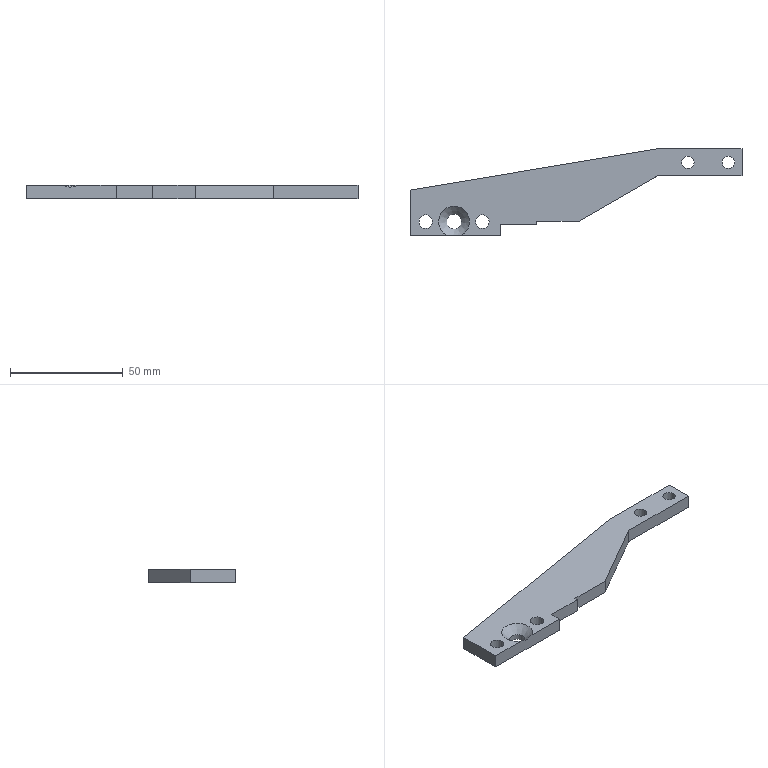Part | NX | features BREP 1 | 1 solid | 19 faces | box 147 x 38.3 x 6 mm | volume 16283 mm3 | plane 13 | cylinder 5 | cone 1 | commonest cylinder face diameters 5.5 x2 6 x2 6.6 x1
STEP:
#1=CARTESIAN_POINT('',(73.5,1.3,-3.));
#2=VERTEX_POINT('',#1);
#3=CARTESIAN_POINT('',(73.5,13.3,-3.));
#4=VERTEX_POINT('',#3);
#5=CARTESIAN_POINT('',(73.5,-25.,-3.));
#6=DIRECTION('',(0.,1.,0.));
#7=VECTOR('',#6,1000.);
#8=LINE('',#5,#7);
#9=EDGE_CURVE('',#2,#4,#8,.T.);
#10=ORIENTED_EDGE('',*,*,#9,.T.);
#11=CARTESIAN_POINT('',(73.5,13.3,3.));
#12=VERTEX_POINT('',#11);
#13=CARTESIAN_POINT('',(73.5,13.3,-153.03));
#14=DIRECTION('',(0.,0.,1.));
#15=VECTOR('',#14,1000.);
#16=LINE('',#13,#15);
#17=EDGE_CURVE('',#4,#12,#16,.T.);
#18=ORIENTED_EDGE('',*,*,#17,.T.);
#19=CARTESIAN_POINT('',(73.5,1.3,3.));
#20=VERTEX_POINT('',#19);
#21=CARTESIAN_POINT('',(73.5,-25.,3.));
#22=DIRECTION('',(0.,1.,0.));
#23=VECTOR('',#22,1000.);
#24=LINE('',#21,#23);
#25=EDGE_CURVE('',#20,#12,#24,.T.);
#26=ORIENTED_EDGE('',*,*,#25,.F.);
#27=CARTESIAN_POINT('',(73.5,1.3,-113.185));
#28=DIRECTION('',(0.,0.,1.));
#29=VECTOR('',#28,1000.);
#30=LINE('',#27,#29);
#31=EDGE_CURVE('',#2,#20,#30,.T.);
#32=ORIENTED_EDGE('',*,*,#31,.F.);
#33=EDGE_LOOP('',(#10,#18,#26,#32));
#34=FACE_BOUND('',#33,.T.);
#35=CARTESIAN_POINT('',(73.5,-25.,3.));
#36=DIRECTION('',(-1.,0.,0.));
#37=DIRECTION('',(0.,0.,-1.));
#38=AXIS2_PLACEMENT_3D('',#35,#36,#37);
#39=PLANE('',#38);
#40=ADVANCED_FACE('',(#34),#39,.F.);
#41=CARTESIAN_POINT('',(-73.5,-5.,3.));
#42=VERTEX_POINT('',#41);
#43=CARTESIAN_POINT('',(-73.5,-25.,3.));
#44=VERTEX_POINT('',#43);
#45=CARTESIAN_POINT('',(-73.5,-25.,3.));
#46=DIRECTION('',(0.,-1.,0.));
#47=VECTOR('',#46,1000.);
#48=LINE('',#45,#47);
#49=EDGE_CURVE('',#42,#44,#48,.T.);
#50=ORIENTED_EDGE('',*,*,#49,.F.);
#51=CARTESIAN_POINT('',(-73.5,-5.,-3.));
#52=VERTEX_POINT('',#51);
#53=CARTESIAN_POINT('',(-73.5,-5.,-153.03));
#54=DIRECTION('',(0.,0.,1.));
#55=VECTOR('',#54,1000.);
#56=LINE('',#53,#55);
#57=EDGE_CURVE('',#52,#42,#56,.T.);
#58=ORIENTED_EDGE('',*,*,#57,.F.);
#59=CARTESIAN_POINT('',(-73.5,-25.,-3.));
#60=VERTEX_POINT('',#59);
#61=CARTESIAN_POINT('',(-73.5,-25.,-3.));
#62=DIRECTION('',(0.,-1.,0.));
#63=VECTOR('',#62,1000.);
#64=LINE('',#61,#63);
#65=EDGE_CURVE('',#52,#60,#64,.T.);
#66=ORIENTED_EDGE('',*,*,#65,.T.);
#67=CARTESIAN_POINT('',(-73.5,-25.,3.));
#68=DIRECTION('',(0.,0.,-1.));
#69=VECTOR('',#68,1000.);
#70=LINE('',#67,#69);
#71=EDGE_CURVE('',#44,#60,#70,.T.);
#72=ORIENTED_EDGE('',*,*,#71,.F.);
#73=EDGE_LOOP('',(#50,#58,#66,#72));
#74=FACE_BOUND('',#73,.T.);
#75=CARTESIAN_POINT('',(-73.5,-25.,3.));
#76=DIRECTION('',(1.,0.,0.));
#77=DIRECTION('',(0.,0.,1.));
#78=AXIS2_PLACEMENT_3D('',#75,#76,#77);
#79=PLANE('',#78);
#80=ADVANCED_FACE('',(#74),#79,.F.);
#81=CARTESIAN_POINT('',(-33.5,-25.,-3.));
#82=VERTEX_POINT('',#81);
#83=CARTESIAN_POINT('',(-73.5,-25.,-3.));
#84=DIRECTION('',(1.,0.,0.));
#85=VECTOR('',#84,1000.);
#86=LINE('',#83,#85);
#87=EDGE_CURVE('',#60,#82,#86,.T.);
#88=ORIENTED_EDGE('',*,*,#87,.T.);
#89=CARTESIAN_POINT('',(-33.5,-25.,3.));
#90=VERTEX_POINT('',#89);
#91=CARTESIAN_POINT('',(-33.5,-25.,-113.185));
#92=DIRECTION('',(0.,0.,1.));
#93=VECTOR('',#92,1000.);
#94=LINE('',#91,#93);
#95=EDGE_CURVE('',#82,#90,#94,.T.);
#96=ORIENTED_EDGE('',*,*,#95,.T.);
#97=CARTESIAN_POINT('',(-50.685,-25.,3.));
#98=VERTEX_POINT('',#97);
#99=CARTESIAN_POINT('',(-73.5,-25.,3.));
#100=DIRECTION('',(1.,0.,0.));
#101=VECTOR('',#100,1000.);
#102=LINE('',#99,#101);
#103=EDGE_CURVE('',#98,#90,#102,.T.);
#104=ORIENTED_EDGE('',*,*,#103,.F.);
#105=CARTESIAN_POINT('',(-57.315,-25.,3.));
#106=VERTEX_POINT('',#105);
#107=CARTESIAN_POINT('',(-50.685,-25.,3.));
#108=CARTESIAN_POINT('',(-51.725,-25.,2.497));
#109=CARTESIAN_POINT('',(-53.981,-25.,1.794));
#110=CARTESIAN_POINT('',(-56.27,-25.,2.494));
#111=CARTESIAN_POINT('',(-57.315,-25.,3.));
#112=B_SPLINE_CURVE_WITH_KNOTS('',3,(#107,#108,#109,#110,#111),.UNSPECIFIED.,.F.,.F.,(4,1,4),(0.,0.003417,0.006834),.UNSPECIFIED.);
#113=EDGE_CURVE('',#98,#106,#112,.T.);
#114=ORIENTED_EDGE('',*,*,#113,.T.);
#115=CARTESIAN_POINT('',(-73.5,-25.,3.));
#116=DIRECTION('',(1.,0.,0.));
#117=VECTOR('',#116,1000.);
#118=LINE('',#115,#117);
#119=EDGE_CURVE('',#44,#106,#118,.T.);
#120=ORIENTED_EDGE('',*,*,#119,.F.);
#121=ORIENTED_EDGE('',*,*,#71,.T.);
#122=EDGE_LOOP('',(#88,#96,#104,#114,#120,#121));
#123=FACE_BOUND('',#122,.T.);
#124=CARTESIAN_POINT('',(-73.5,-25.,3.));
#125=DIRECTION('',(0.,1.,0.));
#126=DIRECTION('',(0.,0.,-1.));
#127=AXIS2_PLACEMENT_3D('',#124,#125,#126);
#128=PLANE('',#127);
#129=ADVANCED_FACE('',(#123),#128,.F.);
#130=CARTESIAN_POINT('',(52.25,7.3,3.));
#131=VERTEX_POINT('',#130);
#132=CARTESIAN_POINT('',(49.5,7.3,3.));
#133=DIRECTION('',(0.,0.,1.));
#134=DIRECTION('',(1.,0.,0.));
#135=AXIS2_PLACEMENT_3D('',#132,#133,#134);
#136=CIRCLE('',#135,2.75);
#137=EDGE_CURVE('',#131,#131,#136,.T.);
#138=ORIENTED_EDGE('',*,*,#137,.F.);
#139=EDGE_LOOP('',(#138));
#140=FACE_BOUND('',#139,.T.);
#141=CARTESIAN_POINT('',(70.25,7.3,3.));
#142=VERTEX_POINT('',#141);
#143=CARTESIAN_POINT('',(67.5,7.3,3.));
#144=DIRECTION('',(0.,0.,1.));
#145=DIRECTION('',(1.,0.,0.));
#146=AXIS2_PLACEMENT_3D('',#143,#144,#145);
#147=CIRCLE('',#146,2.75);
#148=EDGE_CURVE('',#142,#142,#147,.T.);
#149=ORIENTED_EDGE('',*,*,#148,.F.);
#150=EDGE_LOOP('',(#149));
#151=FACE_BOUND('',#150,.T.);
#152=CARTESIAN_POINT('',(-63.5,-19.,3.));
#153=VERTEX_POINT('',#152);
#154=CARTESIAN_POINT('',(-66.5,-19.,3.));
#155=DIRECTION('',(0.,0.,1.));
#156=DIRECTION('',(1.,0.,0.));
#157=AXIS2_PLACEMENT_3D('',#154,#155,#156);
#158=CIRCLE('',#157,3.);
#159=EDGE_CURVE('',#153,#153,#158,.T.);
#160=ORIENTED_EDGE('',*,*,#159,.F.);
#161=EDGE_LOOP('',(#160));
#162=FACE_BOUND('',#161,.T.);
#163=CARTESIAN_POINT('',(-38.5,-19.,3.));
#164=VERTEX_POINT('',#163);
#165=CARTESIAN_POINT('',(-41.5,-19.,3.));
#166=DIRECTION('',(0.,0.,1.));
#167=DIRECTION('',(1.,0.,0.));
#168=AXIS2_PLACEMENT_3D('',#165,#166,#167);
#169=CIRCLE('',#168,3.);
#170=EDGE_CURVE('',#164,#164,#169,.T.);
#171=ORIENTED_EDGE('',*,*,#170,.F.);
#172=EDGE_LOOP('',(#171));
#173=FACE_BOUND('',#172,.T.);
#174=CARTESIAN_POINT('',(36.141,13.3,3.));
#175=VERTEX_POINT('',#174);
#176=CARTESIAN_POINT('',(36.141,13.3,3.));
#177=DIRECTION('',(1.,0.,0.));
#178=VECTOR('',#177,1000.);
#179=LINE('',#176,#178);
#180=EDGE_CURVE('',#175,#12,#179,.T.);
#181=ORIENTED_EDGE('',*,*,#180,.F.);
#182=CARTESIAN_POINT('',(-73.5,-5.,3.));
#183=DIRECTION('',(0.9864,0.1646,0.));
#184=VECTOR('',#183,1000.);
#185=LINE('',#182,#184);
#186=EDGE_CURVE('',#42,#175,#185,.T.);
#187=ORIENTED_EDGE('',*,*,#186,.F.);
#188=ORIENTED_EDGE('',*,*,#49,.T.);
#189=ORIENTED_EDGE('',*,*,#119,.T.);
#190=CARTESIAN_POINT('',(-54.,-19.,3.));
#191=DIRECTION('',(0.,0.,1.));
#192=DIRECTION('',(1.,0.,0.));
#193=AXIS2_PLACEMENT_3D('',#190,#191,#192);
#194=CIRCLE('',#193,6.855);
#195=EDGE_CURVE('',#98,#106,#194,.T.);
#196=ORIENTED_EDGE('',*,*,#195,.F.);
#197=ORIENTED_EDGE('',*,*,#103,.T.);
#198=CARTESIAN_POINT('',(-33.5,-20.1,3.));
#199=VERTEX_POINT('',#198);
#200=CARTESIAN_POINT('',(-33.5,-25.,3.));
#201=DIRECTION('',(0.,-1.,0.));
#202=VECTOR('',#201,1000.);
#203=LINE('',#200,#202);
#204=EDGE_CURVE('',#199,#90,#203,.T.);
#205=ORIENTED_EDGE('',*,*,#204,.F.);
#206=CARTESIAN_POINT('',(-17.5,-20.1,3.));
#207=VERTEX_POINT('',#206);
#208=CARTESIAN_POINT('',(-33.5,-20.1,3.));
#209=DIRECTION('',(1.,0.,0.));
#210=VECTOR('',#209,1000.);
#211=LINE('',#208,#210);
#212=EDGE_CURVE('',#199,#207,#211,.T.);
#213=ORIENTED_EDGE('',*,*,#212,.T.);
#214=CARTESIAN_POINT('',(-17.5,-18.7,3.));
#215=VERTEX_POINT('',#214);
#216=CARTESIAN_POINT('',(-17.5,-18.7,3.));
#217=DIRECTION('',(0.,1.,0.));
#218=VECTOR('',#217,1000.);
#219=LINE('',#216,#218);
#220=EDGE_CURVE('',#207,#215,#219,.T.);
#221=ORIENTED_EDGE('',*,*,#220,.T.);
#222=CARTESIAN_POINT('',(1.5,-18.7,3.));
#223=VERTEX_POINT('',#222);
#224=CARTESIAN_POINT('',(-33.5,-18.7,3.));
#225=DIRECTION('',(-1.,0.,0.));
#226=VECTOR('',#225,1000.);
#227=LINE('',#224,#226);
#228=EDGE_CURVE('',#223,#215,#227,.T.);
#229=ORIENTED_EDGE('',*,*,#228,.F.);
#230=CARTESIAN_POINT('',(36.141,1.3,3.));
#231=VERTEX_POINT('',#230);
#232=CARTESIAN_POINT('',(1.5,-18.7,3.));
#233=DIRECTION('',(-0.866,-0.5,0.));
#234=VECTOR('',#233,1000.);
#235=LINE('',#232,#234);
#236=EDGE_CURVE('',#231,#223,#235,.T.);
#237=ORIENTED_EDGE('',*,*,#236,.F.);
#238=CARTESIAN_POINT('',(36.141,1.3,3.));
#239=DIRECTION('',(-1.,0.,0.));
#240=VECTOR('',#239,1000.);
#241=LINE('',#238,#240);
#242=EDGE_CURVE('',#20,#231,#241,.T.);
#243=ORIENTED_EDGE('',*,*,#242,.F.);
#244=ORIENTED_EDGE('',*,*,#25,.T.);
#245=EDGE_LOOP('',(#181,#187,#188,#189,#196,#197,#205,#213,#221,#229,#237,#243,#244));
#246=FACE_BOUND('',#245,.T.);
#247=CARTESIAN_POINT('',(0.,0.,3.));
#248=DIRECTION('',(0.,0.,-1.));
#249=DIRECTION('',(1.,0.,0.));
#250=AXIS2_PLACEMENT_3D('',#247,#248,#249);
#251=PLANE('',#250);
#252=ADVANCED_FACE('',(#140,#151,#162,#173,#246),#251,.F.);
#253=CARTESIAN_POINT('',(46.75,7.3,-3.));
#254=VERTEX_POINT('',#253);
#255=CARTESIAN_POINT('',(49.5,7.3,-3.));
#256=DIRECTION('',(0.,0.,-1.));
#257=DIRECTION('',(-1.,0.,0.));
#258=AXIS2_PLACEMENT_3D('',#255,#256,#257);
#259=CIRCLE('',#258,2.75);
#260=EDGE_CURVE('',#254,#254,#259,.T.);
#261=ORIENTED_EDGE('',*,*,#260,.F.);
#262=EDGE_LOOP('',(#261));
#263=FACE_BOUND('',#262,.T.);
#264=CARTESIAN_POINT('',(64.75,7.3,-3.));
#265=VERTEX_POINT('',#264);
#266=CARTESIAN_POINT('',(67.5,7.3,-3.));
#267=DIRECTION('',(0.,0.,-1.));
#268=DIRECTION('',(-1.,0.,0.));
#269=AXIS2_PLACEMENT_3D('',#266,#267,#268);
#270=CIRCLE('',#269,2.75);
#271=EDGE_CURVE('',#265,#265,#270,.T.);
#272=ORIENTED_EDGE('',*,*,#271,.F.);
#273=EDGE_LOOP('',(#272));
#274=FACE_BOUND('',#273,.T.);
#275=CARTESIAN_POINT('',(36.141,13.3,-3.));
#276=VERTEX_POINT('',#275);
#277=CARTESIAN_POINT('',(-73.5,-5.,-3.));
#278=DIRECTION('',(0.9864,0.1646,0.));
#279=VECTOR('',#278,1000.);
#280=LINE('',#277,#279);
#281=EDGE_CURVE('',#52,#276,#280,.T.);
#282=ORIENTED_EDGE('',*,*,#281,.T.);
#283=CARTESIAN_POINT('',(36.141,13.3,-3.));
#284=DIRECTION('',(1.,0.,0.));
#285=VECTOR('',#284,1000.);
#286=LINE('',#283,#285);
#287=EDGE_CURVE('',#276,#4,#286,.T.);
#288=ORIENTED_EDGE('',*,*,#287,.T.);
#289=ORIENTED_EDGE('',*,*,#9,.F.);
#290=CARTESIAN_POINT('',(36.141,1.3,-3.));
#291=VERTEX_POINT('',#290);
#292=CARTESIAN_POINT('',(36.141,1.3,-3.));
#293=DIRECTION('',(-1.,0.,0.));
#294=VECTOR('',#293,1000.);
#295=LINE('',#292,#294);
#296=EDGE_CURVE('',#2,#291,#295,.T.);
#297=ORIENTED_EDGE('',*,*,#296,.T.);
#298=CARTESIAN_POINT('',(1.5,-18.7,-3.));
#299=VERTEX_POINT('',#298);
#300=CARTESIAN_POINT('',(1.5,-18.7,-3.));
#301=DIRECTION('',(-0.866,-0.5,0.));
#302=VECTOR('',#301,1000.);
#303=LINE('',#300,#302);
#304=EDGE_CURVE('',#291,#299,#303,.T.);
#305=ORIENTED_EDGE('',*,*,#304,.T.);
#306=CARTESIAN_POINT('',(-17.5,-18.7,-3.));
#307=VERTEX_POINT('',#306);
#308=CARTESIAN_POINT('',(-33.5,-18.7,-3.));
#309=DIRECTION('',(-1.,0.,0.));
#310=VECTOR('',#309,1000.);
#311=LINE('',#308,#310);
#312=EDGE_CURVE('',#299,#307,#311,.T.);
#313=ORIENTED_EDGE('',*,*,#312,.T.);
#314=CARTESIAN_POINT('',(-17.5,-20.1,-3.));
#315=VERTEX_POINT('',#314);
#316=CARTESIAN_POINT('',(-17.5,-18.7,-3.));
#317=DIRECTION('',(0.,1.,0.));
#318=VECTOR('',#317,1000.);
#319=LINE('',#316,#318);
#320=EDGE_CURVE('',#315,#307,#319,.T.);
#321=ORIENTED_EDGE('',*,*,#320,.F.);
#322=CARTESIAN_POINT('',(-33.5,-20.1,-3.));
#323=VERTEX_POINT('',#322);
#324=CARTESIAN_POINT('',(-33.5,-20.1,-3.));
#325=DIRECTION('',(1.,0.,0.));
#326=VECTOR('',#325,1000.);
#327=LINE('',#324,#326);
#328=EDGE_CURVE('',#323,#315,#327,.T.);
#329=ORIENTED_EDGE('',*,*,#328,.F.);
#330=CARTESIAN_POINT('',(-33.5,-25.,-3.));
#331=DIRECTION('',(0.,-1.,0.));
#332=VECTOR('',#331,1000.);
#333=LINE('',#330,#332);
#334=EDGE_CURVE('',#323,#82,#333,.T.);
#335=ORIENTED_EDGE('',*,*,#334,.T.);
#336=ORIENTED_EDGE('',*,*,#87,.F.);
#337=ORIENTED_EDGE('',*,*,#65,.F.);
#338=EDGE_LOOP('',(#282,#288,#289,#297,#305,#313,#321,#329,#335,#336,#337));
#339=FACE_BOUND('',#338,.T.);
#340=CARTESIAN_POINT('',(-50.7,-19.,-3.));
#341=VERTEX_POINT('',#340);
#342=CARTESIAN_POINT('',(-54.,-19.,-3.));
#343=DIRECTION('',(0.,0.,1.));
#344=DIRECTION('',(1.,0.,0.));
#345=AXIS2_PLACEMENT_3D('',#342,#343,#344);
#346=CIRCLE('',#345,3.3);
#347=EDGE_CURVE('',#341,#341,#346,.T.);
#348=ORIENTED_EDGE('',*,*,#347,.T.);
#349=EDGE_LOOP('',(#348));
#350=FACE_BOUND('',#349,.T.);
#351=CARTESIAN_POINT('',(-63.5,-19.,-3.));
#352=VERTEX_POINT('',#351);
#353=CARTESIAN_POINT('',(-66.5,-19.,-3.));
#354=DIRECTION('',(0.,0.,1.));
#355=DIRECTION('',(1.,0.,0.));
#356=AXIS2_PLACEMENT_3D('',#353,#354,#355);
#357=CIRCLE('',#356,3.);
#358=EDGE_CURVE('',#352,#352,#357,.T.);
#359=ORIENTED_EDGE('',*,*,#358,.T.);
#360=EDGE_LOOP('',(#359));
#361=FACE_BOUND('',#360,.T.);
#362=CARTESIAN_POINT('',(-38.5,-19.,-3.));
#363=VERTEX_POINT('',#362);
#364=CARTESIAN_POINT('',(-41.5,-19.,-3.));
#365=DIRECTION('',(0.,0.,1.));
#366=DIRECTION('',(1.,0.,0.));
#367=AXIS2_PLACEMENT_3D('',#364,#365,#366);
#368=CIRCLE('',#367,3.);
#369=EDGE_CURVE('',#363,#363,#368,.T.);
#370=ORIENTED_EDGE('',*,*,#369,.T.);
#371=EDGE_LOOP('',(#370));
#372=FACE_BOUND('',#371,.T.);
#373=CARTESIAN_POINT('',(0.,0.,-3.));
#374=DIRECTION('',(0.,0.,-1.));
#375=DIRECTION('',(1.,0.,0.));
#376=AXIS2_PLACEMENT_3D('',#373,#374,#375);
#377=PLANE('',#376);
#378=ADVANCED_FACE('',(#263,#274,#339,#350,#361,#372),#377,.T.);
#379=ORIENTED_EDGE('',*,*,#369,.F.);
#380=EDGE_LOOP('',(#379));
#381=FACE_BOUND('',#380,.T.);
#382=ORIENTED_EDGE('',*,*,#170,.T.);
#383=EDGE_LOOP('',(#382));
#384=FACE_BOUND('',#383,.T.);
#385=CARTESIAN_POINT('',(-41.5,-19.,3.));
#386=DIRECTION('',(0.,0.,1.));
#387=DIRECTION('',(-1.,0.,0.));
#388=AXIS2_PLACEMENT_3D('',#385,#386,#387);
#389=CYLINDRICAL_SURFACE('',#388,3.);
#390=ADVANCED_FACE('',(#381,#384),#389,.F.);
#391=ORIENTED_EDGE('',*,*,#358,.F.);
#392=EDGE_LOOP('',(#391));
#393=FACE_BOUND('',#392,.T.);
#394=ORIENTED_EDGE('',*,*,#159,.T.);
#395=EDGE_LOOP('',(#394));
#396=FACE_BOUND('',#395,.T.);
#397=CARTESIAN_POINT('',(-66.5,-19.,3.));
#398=DIRECTION('',(0.,0.,1.));
#399=DIRECTION('',(-1.,0.,0.));
#400=AXIS2_PLACEMENT_3D('',#397,#398,#399);
#401=CYLINDRICAL_SURFACE('',#400,3.);
#402=ADVANCED_FACE('',(#393,#396),#401,.F.);
#403=CARTESIAN_POINT('',(-50.7,-19.,-0.555));
#404=VERTEX_POINT('',#403);
#405=CARTESIAN_POINT('',(-54.,-19.,-0.555));
#406=DIRECTION('',(0.,0.,1.));
#407=DIRECTION('',(1.,0.,0.));
#408=AXIS2_PLACEMENT_3D('',#405,#406,#407);
#409=CIRCLE('',#408,3.3);
#410=EDGE_CURVE('',#404,#404,#409,.T.);
#411=ORIENTED_EDGE('',*,*,#410,.F.);
#412=EDGE_LOOP('',(#411));
#413=FACE_BOUND('',#412,.T.);
#414=ORIENTED_EDGE('',*,*,#195,.T.);
#415=ORIENTED_EDGE('',*,*,#113,.F.);
#416=EDGE_LOOP('',(#414,#415));
#417=FACE_BOUND('',#416,.T.);
#418=CARTESIAN_POINT('',(-54.,-19.,3.));
#419=DIRECTION('',(0.,0.,1.));
#420=DIRECTION('',(-1.,0.,0.));
#421=AXIS2_PLACEMENT_3D('',#418,#419,#420);
#422=CONICAL_SURFACE('',#421,6.855,0.7854);
#423=ADVANCED_FACE('',(#413,#417),#422,.F.);
#424=ORIENTED_EDGE('',*,*,#347,.F.);
#425=EDGE_LOOP('',(#424));
#426=FACE_BOUND('',#425,.T.);
#427=ORIENTED_EDGE('',*,*,#410,.T.);
#428=EDGE_LOOP('',(#427));
#429=FACE_BOUND('',#428,.T.);
#430=CARTESIAN_POINT('',(-54.,-19.,3.));
#431=DIRECTION('',(0.,0.,1.));
#432=DIRECTION('',(-1.,0.,0.));
#433=AXIS2_PLACEMENT_3D('',#430,#431,#432);
#434=CYLINDRICAL_SURFACE('',#433,3.3);
#435=ADVANCED_FACE('',(#426,#429),#434,.F.);
#436=ORIENTED_EDGE('',*,*,#31,.T.);
#437=ORIENTED_EDGE('',*,*,#242,.T.);
#438=CARTESIAN_POINT('',(36.141,1.3,-113.185));
#439=DIRECTION('',(0.,0.,1.));
#440=VECTOR('',#439,1000.);
#441=LINE('',#438,#440);
#442=EDGE_CURVE('',#291,#231,#441,.T.);
#443=ORIENTED_EDGE('',*,*,#442,.F.);
#444=ORIENTED_EDGE('',*,*,#296,.F.);
#445=EDGE_LOOP('',(#436,#437,#443,#444));
#446=FACE_BOUND('',#445,.T.);
#447=CARTESIAN_POINT('',(36.141,1.3,-113.185));
#448=DIRECTION('',(0.,1.,0.));
#449=DIRECTION('',(0.,0.,-1.));
#450=AXIS2_PLACEMENT_3D('',#447,#448,#449);
#451=PLANE('',#450);
#452=ADVANCED_FACE('',(#446),#451,.F.);
#453=ORIENTED_EDGE('',*,*,#442,.T.);
#454=ORIENTED_EDGE('',*,*,#236,.T.);
#455=CARTESIAN_POINT('',(1.5,-18.7,-113.185));
#456=DIRECTION('',(0.,0.,1.));
#457=VECTOR('',#456,1000.);
#458=LINE('',#455,#457);
#459=EDGE_CURVE('',#299,#223,#458,.T.);
#460=ORIENTED_EDGE('',*,*,#459,.F.);
#461=ORIENTED_EDGE('',*,*,#304,.F.);
#462=EDGE_LOOP('',(#453,#454,#460,#461));
#463=FACE_BOUND('',#462,.T.);
#464=CARTESIAN_POINT('',(1.5,-18.7,-113.185));
#465=DIRECTION('',(-0.5,0.866,0.));
#466=DIRECTION('',(0.866,0.5,0.));
#467=AXIS2_PLACEMENT_3D('',#464,#465,#466);
#468=PLANE('',#467);
#469=ADVANCED_FACE('',(#463),#468,.F.);
#470=ORIENTED_EDGE('',*,*,#228,.T.);
#471=CARTESIAN_POINT('',(-17.5,-18.7,-19.061));
#472=DIRECTION('',(0.,0.,1.));
#473=VECTOR('',#472,1000.);
#474=LINE('',#471,#473);
#475=EDGE_CURVE('',#307,#215,#474,.T.);
#476=ORIENTED_EDGE('',*,*,#475,.F.);
#477=ORIENTED_EDGE('',*,*,#312,.F.);
#478=ORIENTED_EDGE('',*,*,#459,.T.);
#479=EDGE_LOOP('',(#470,#476,#477,#478));
#480=FACE_BOUND('',#479,.T.);
#481=CARTESIAN_POINT('',(-33.5,-18.7,-113.185));
#482=DIRECTION('',(0.,1.,0.));
#483=DIRECTION('',(0.,0.,-1.));
#484=AXIS2_PLACEMENT_3D('',#481,#482,#483);
#485=PLANE('',#484);
#486=ADVANCED_FACE('',(#480),#485,.F.);
#487=ORIENTED_EDGE('',*,*,#334,.F.);
#488=CARTESIAN_POINT('',(-33.5,-20.1,-19.061));
#489=DIRECTION('',(0.,0.,1.));
#490=VECTOR('',#489,1000.);
#491=LINE('',#488,#490);
#492=EDGE_CURVE('',#323,#199,#491,.T.);
#493=ORIENTED_EDGE('',*,*,#492,.T.);
#494=ORIENTED_EDGE('',*,*,#204,.T.);
#495=ORIENTED_EDGE('',*,*,#95,.F.);
#496=EDGE_LOOP('',(#487,#493,#494,#495));
#497=FACE_BOUND('',#496,.T.);
#498=CARTESIAN_POINT('',(-33.5,-25.,-113.185));
#499=DIRECTION('',(-1.,0.,0.));
#500=DIRECTION('',(0.,0.,-1.));
#501=AXIS2_PLACEMENT_3D('',#498,#499,#500);
#502=PLANE('',#501);
#503=ADVANCED_FACE('',(#497),#502,.F.);
#504=ORIENTED_EDGE('',*,*,#57,.T.);
#505=ORIENTED_EDGE('',*,*,#186,.T.);
#506=CARTESIAN_POINT('',(36.141,13.3,-153.03));
#507=DIRECTION('',(0.,0.,1.));
#508=VECTOR('',#507,1000.);
#509=LINE('',#506,#508);
#510=EDGE_CURVE('',#276,#175,#509,.T.);
#511=ORIENTED_EDGE('',*,*,#510,.F.);
#512=ORIENTED_EDGE('',*,*,#281,.F.);
#513=EDGE_LOOP('',(#504,#505,#511,#512));
#514=FACE_BOUND('',#513,.T.);
#515=CARTESIAN_POINT('',(-73.5,-5.,-153.03));
#516=DIRECTION('',(0.1646,-0.9864,0.));
#517=DIRECTION('',(-0.9864,-0.1646,0.));
#518=AXIS2_PLACEMENT_3D('',#515,#516,#517);
#519=PLANE('',#518);
#520=ADVANCED_FACE('',(#514),#519,.F.);
#521=ORIENTED_EDGE('',*,*,#510,.T.);
#522=ORIENTED_EDGE('',*,*,#180,.T.);
#523=ORIENTED_EDGE('',*,*,#17,.F.);
#524=ORIENTED_EDGE('',*,*,#287,.F.);
#525=EDGE_LOOP('',(#521,#522,#523,#524));
#526=FACE_BOUND('',#525,.T.);
#527=CARTESIAN_POINT('',(36.141,13.3,-153.03));
#528=DIRECTION('',(0.,-1.,0.));
#529=DIRECTION('',(0.,0.,1.));
#530=AXIS2_PLACEMENT_3D('',#527,#528,#529);
#531=PLANE('',#530);
#532=ADVANCED_FACE('',(#526),#531,.F.);
#533=ORIENTED_EDGE('',*,*,#271,.T.);
#534=EDGE_LOOP('',(#533));
#535=FACE_BOUND('',#534,.T.);
#536=ORIENTED_EDGE('',*,*,#148,.T.);
#537=EDGE_LOOP('',(#536));
#538=FACE_BOUND('',#537,.T.);
#539=CARTESIAN_POINT('',(67.5,7.3,3.));
#540=DIRECTION('',(0.,0.,1.));
#541=DIRECTION('',(-1.,0.,0.));
#542=AXIS2_PLACEMENT_3D('',#539,#540,#541);
#543=CYLINDRICAL_SURFACE('',#542,2.75);
#544=ADVANCED_FACE('',(#535,#538),#543,.F.);
#545=ORIENTED_EDGE('',*,*,#260,.T.);
#546=EDGE_LOOP('',(#545));
#547=FACE_BOUND('',#546,.T.);
#548=ORIENTED_EDGE('',*,*,#137,.T.);
#549=EDGE_LOOP('',(#548));
#550=FACE_BOUND('',#549,.T.);
#551=CARTESIAN_POINT('',(49.5,7.3,3.));
#552=DIRECTION('',(0.,0.,1.));
#553=DIRECTION('',(-1.,0.,0.));
#554=AXIS2_PLACEMENT_3D('',#551,#552,#553);
#555=CYLINDRICAL_SURFACE('',#554,2.75);
#556=ADVANCED_FACE('',(#547,#550),#555,.F.);
#557=ORIENTED_EDGE('',*,*,#492,.F.);
#558=ORIENTED_EDGE('',*,*,#328,.T.);
#559=CARTESIAN_POINT('',(-17.5,-20.1,-19.061));
#560=DIRECTION('',(0.,0.,1.));
#561=VECTOR('',#560,1000.);
#562=LINE('',#559,#561);
#563=EDGE_CURVE('',#315,#207,#562,.T.);
#564=ORIENTED_EDGE('',*,*,#563,.T.);
#565=ORIENTED_EDGE('',*,*,#212,.F.);
#566=EDGE_LOOP('',(#557,#558,#564,#565));
#567=FACE_BOUND('',#566,.T.);
#568=CARTESIAN_POINT('',(-33.5,-20.1,-19.061));
#569=DIRECTION('',(0.,-1.,0.));
#570=DIRECTION('',(0.,0.,1.));
#571=AXIS2_PLACEMENT_3D('',#568,#569,#570);
#572=PLANE('',#571);
#573=ADVANCED_FACE('',(#567),#572,.T.);
#574=ORIENTED_EDGE('',*,*,#563,.F.);
#575=ORIENTED_EDGE('',*,*,#320,.T.);
#576=ORIENTED_EDGE('',*,*,#475,.T.);
#577=ORIENTED_EDGE('',*,*,#220,.F.);
#578=EDGE_LOOP('',(#574,#575,#576,#577));
#579=FACE_BOUND('',#578,.T.);
#580=CARTESIAN_POINT('',(-17.5,-18.7,-19.061));
#581=DIRECTION('',(1.,0.,0.));
#582=DIRECTION('',(0.,0.,1.));
#583=AXIS2_PLACEMENT_3D('',#580,#581,#582);
#584=PLANE('',#583);
#585=ADVANCED_FACE('',(#579),#584,.T.);
#586=CLOSED_SHELL('',(#40,#80,#129,#252,#378,#390,#402,#423,#435,#452,#469,#486,#503,#520,#532,#544,#556,#573,#585));
#587=MANIFOLD_SOLID_BREP('',#586);
#588=(LENGTH_UNIT()NAMED_UNIT(*)SI_UNIT(.MILLI.,.METRE.));
#589=UNCERTAINTY_MEASURE_WITH_UNIT(LENGTH_MEASURE(0.0508),#588,'','');
#590=(NAMED_UNIT(*)PLANE_ANGLE_UNIT()SI_UNIT($,.RADIAN.));
#591=(NAMED_UNIT(*)SI_UNIT($,.STERADIAN.)SOLID_ANGLE_UNIT());
#592=(GEOMETRIC_REPRESENTATION_CONTEXT(3)GLOBAL_UNCERTAINTY_ASSIGNED_CONTEXT((#589))GLOBAL_UNIT_ASSIGNED_CONTEXT((#588,#590,#591))REPRESENTATION_CONTEXT('',''));
#593=ADVANCED_BREP_SHAPE_REPRESENTATION('',(#587),#592);